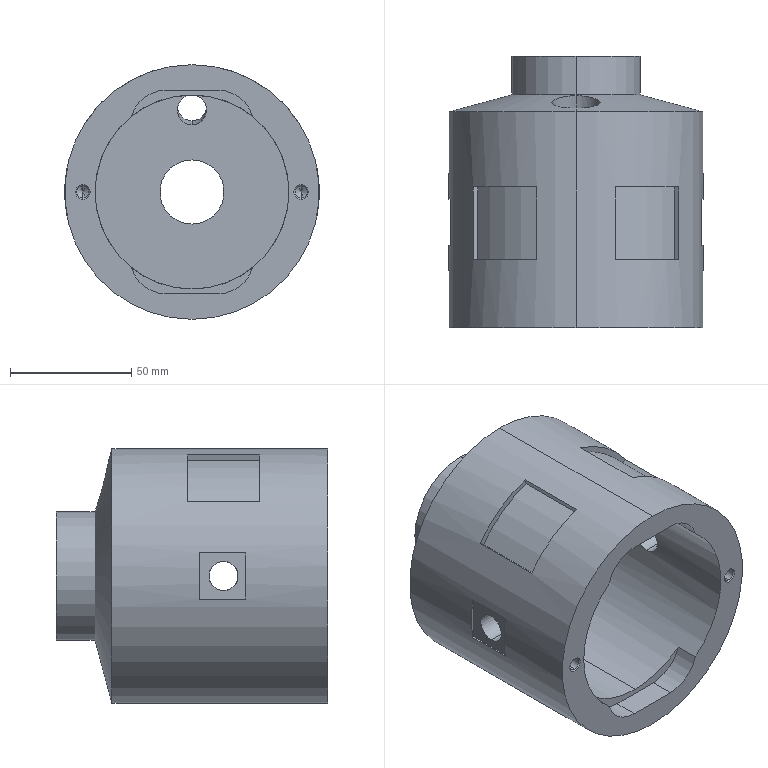Part | SolidWorks | features ICE 5, HoleWzd 2, MirrorPattern 1, RevCut 1, Revolution 1 | 1 solid | 64 faces | box 105 x 112 x 105 mm | volume 406446 mm3 | cylinder 26 | plane 26 | cone 12 | commonest cylinder face diameters 12 x6 5 x4 30 x4 20 x2 26.5 x2 53 x2